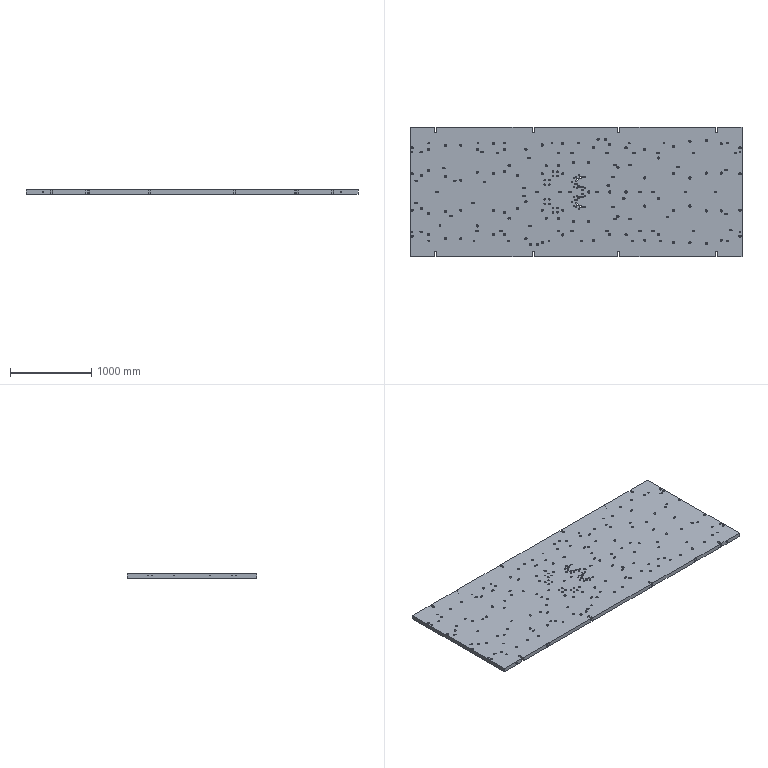Part | NX | features solid 2 | 1 solid | 979 faces | box 4080 x 1595 x 50 mm | volume 320197612 mm3 | cylinder 615 | plane 288 | cone 76 | commonest cylinder face diameters 14.5 x134 18 x128 9 x120 27 x92 8.5 x32 14.1 x20